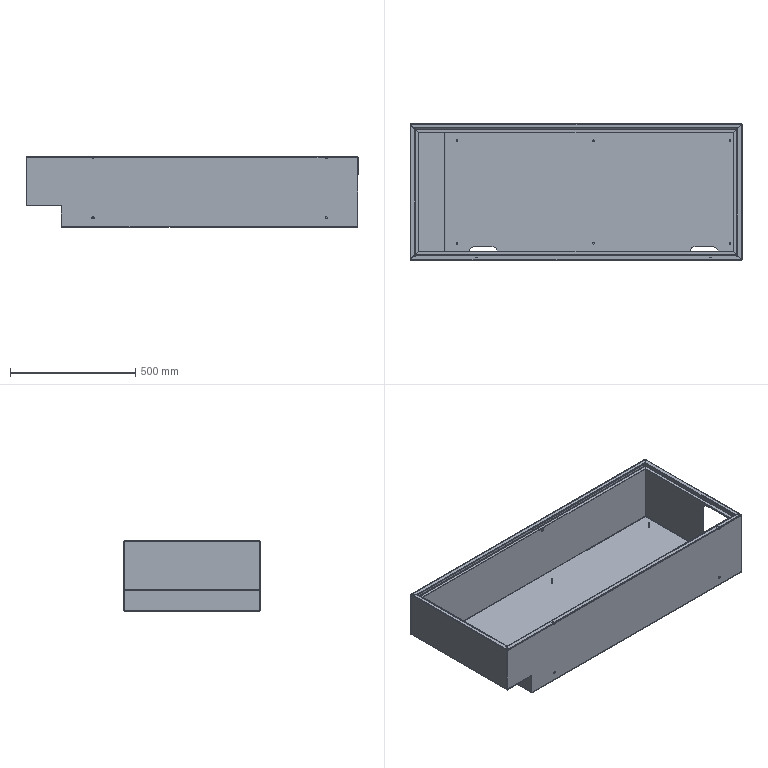Part | SolidWorks | features BaseBody 3 | 3 solids | 252 faces | box 1324 x 545 x 280 mm | volume 3692641 mm3 | plane 136 | cylinder 94 | spline 20 | cone 2 | commonest cylinder face diameters 6 x32 2 x24 9 x10 40 x10 3.3 x8 4 x4